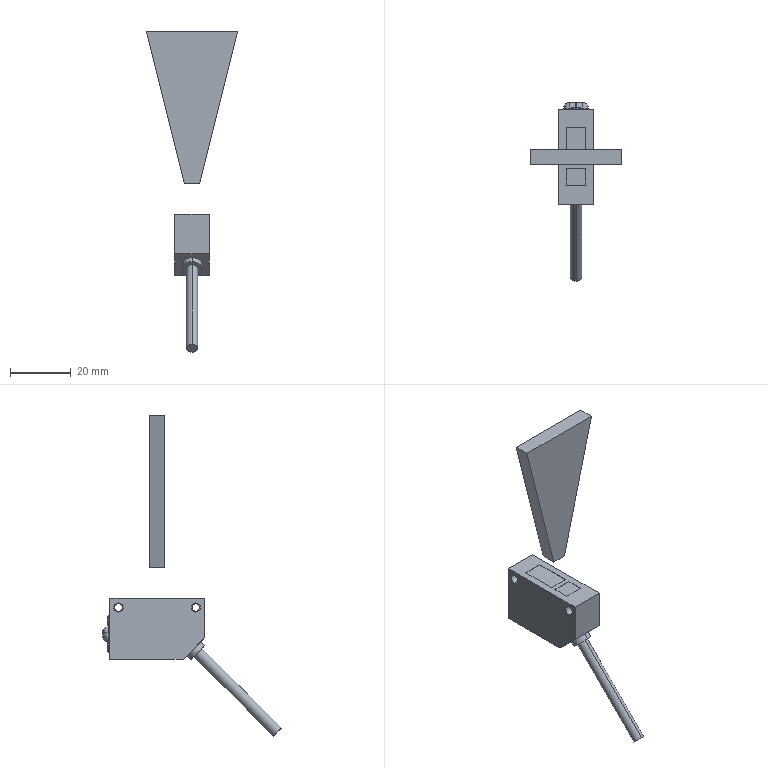Part | STEP file | Retro-reflective photoelectric switch CX-462A | 4 solids | 98 faces | box 30 x 58.715 x 105.315 mm | volume 11448 mm3 | plane 55 | cylinder 32 | cone 7 | sphere 4 | commonest cylinder face diameters 3.6 x10 3 x8 2.5 x4 2.92 x4 3.4 x2 3.7 x2